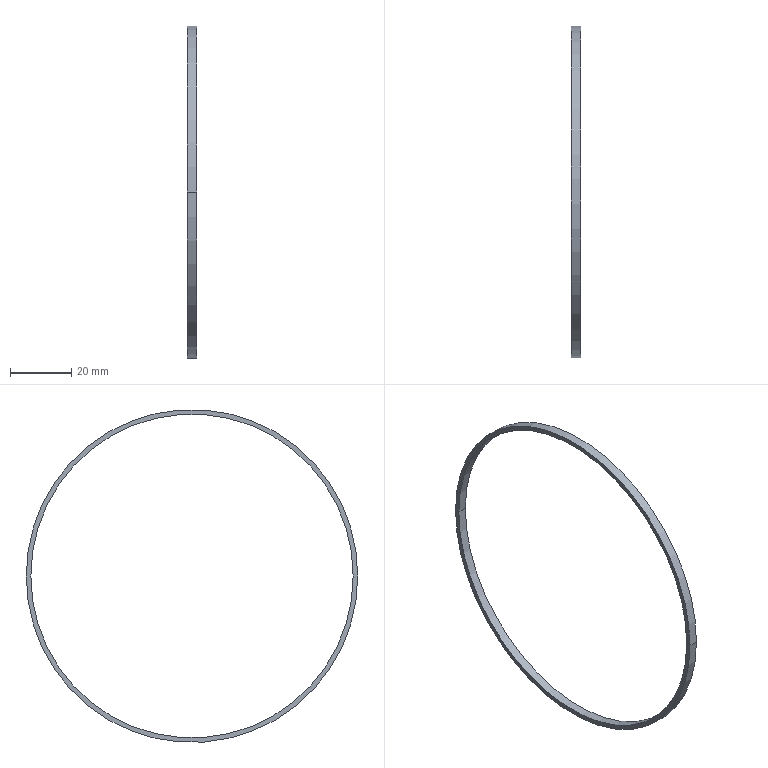Part | STEP file | 1-56.27 | 1 solid | 6 faces | box 3 x 108 x 108.5 mm | volume 1510 mm3 | cylinder 4 | plane 2 | commonest cylinder face diameters 105 x2 108 x2
STEP:
#1=CARTESIAN_POINT('',(0.,0.,0.));
#2=DIRECTION('',(0.,0.,1.));
#3=DIRECTION('',(1.,0.,0.));
#4=AXIS2_PLACEMENT_3D('',#1,#2,#3);
#5=CARTESIAN_POINT('',(0.,53.999,-0.25));
#6=VERTEX_POINT('',#5);
#7=CARTESIAN_POINT('',(0.,-53.999,-0.25));
#8=VERTEX_POINT('',#7);
#9=CARTESIAN_POINT('',(0.,0.,0.));
#10=DIRECTION('',(1.,0.,0.));
#11=DIRECTION('',(0.,1.,-0.00463));
#12=AXIS2_PLACEMENT_3D('',#9,#10,#11);
#13=CIRCLE('',#12,54.);
#14=CARTESIAN_POINT('',(0.,0.,-0.2494));
#15=DIRECTION('',(1.,0.,0.));
#16=DIRECTION('',(0.,1.,0.));
#17=AXIS2_PLACEMENT_3D('',#14,#15,#16);
#18=PLANE('',#17);
#19=CARTESIAN_POINT('',(0.,0.2494));
#20=DIRECTION('',(1.,-0.00463));
#21=AXIS2_PLACEMENT_2D('',#19,#20);
#22=CIRCLE('',#21,54.);
#23=(GEOMETRIC_REPRESENTATION_CONTEXT(2)PARAMETRIC_REPRESENTATION_CONTEXT()REPRESENTATION_CONTEXT('',''));
#24=DEFINITIONAL_REPRESENTATION('',(#22),#23);
#25=PCURVE('',#18,#24);
#26=CARTESIAN_POINT('',(0.,0.,0.));
#27=DIRECTION('',(1.,0.,0.));
#28=DIRECTION('',(0.,1.,-0.00463));
#29=AXIS2_PLACEMENT_3D('',#26,#27,#28);
#30=CYLINDRICAL_SURFACE('',#29,54.);
#31=CARTESIAN_POINT('',(0.,0.));
#32=DIRECTION('',(1.,0.));
#33=VECTOR('',#32,1.);
#34=LINE('',#31,#33);
#35=(GEOMETRIC_REPRESENTATION_CONTEXT(2)PARAMETRIC_REPRESENTATION_CONTEXT()REPRESENTATION_CONTEXT('',''));
#36=DEFINITIONAL_REPRESENTATION('',(#34),#35);
#37=PCURVE('',#30,#36);
#38=SURFACE_CURVE('',#13,(#25,#37),.PCURVE_S1.);
#39=EDGE_CURVE('',#6,#8,#38,.T.);
#40=ORIENTED_EDGE('',*,*,#39,.T.);
#41=CARTESIAN_POINT('',(0.,0.,-0.5));
#42=DIRECTION('',(1.,0.,0.));
#43=DIRECTION('',(0.,-1.,0.00463));
#44=AXIS2_PLACEMENT_3D('',#41,#42,#43);
#45=CIRCLE('',#44,54.);
#46=CARTESIAN_POINT('',(0.,-0.2506));
#47=DIRECTION('',(-1.,0.00463));
#48=AXIS2_PLACEMENT_2D('',#46,#47);
#49=CIRCLE('',#48,54.);
#50=(GEOMETRIC_REPRESENTATION_CONTEXT(2)PARAMETRIC_REPRESENTATION_CONTEXT()REPRESENTATION_CONTEXT('',''));
#51=DEFINITIONAL_REPRESENTATION('',(#49),#50);
#52=PCURVE('',#18,#51);
#53=CARTESIAN_POINT('',(0.,0.,-0.5));
#54=DIRECTION('',(1.,0.,0.));
#55=DIRECTION('',(0.,-1.,0.00463));
#56=AXIS2_PLACEMENT_3D('',#53,#54,#55);
#57=CYLINDRICAL_SURFACE('',#56,54.);
#58=CARTESIAN_POINT('',(0.,0.));
#59=DIRECTION('',(1.,0.));
#60=VECTOR('',#59,1.);
#61=LINE('',#58,#60);
#62=(GEOMETRIC_REPRESENTATION_CONTEXT(2)PARAMETRIC_REPRESENTATION_CONTEXT()REPRESENTATION_CONTEXT('',''));
#63=DEFINITIONAL_REPRESENTATION('',(#61),#62);
#64=PCURVE('',#57,#63);
#65=SURFACE_CURVE('',#45,(#52,#64),.PCURVE_S1.);
#66=EDGE_CURVE('',#8,#6,#65,.T.);
#67=ORIENTED_EDGE('',*,*,#66,.T.);
#68=EDGE_LOOP('',(#40,#67));
#69=FACE_BOUND('',#68,.F.);
#70=CARTESIAN_POINT('',(0.,52.499,-0.25));
#71=VERTEX_POINT('',#70);
#72=CARTESIAN_POINT('',(0.,-52.499,-0.25));
#73=VERTEX_POINT('',#72);
#74=CARTESIAN_POINT('',(0.,0.,-0.5));
#75=DIRECTION('',(-1.,0.,0.));
#76=DIRECTION('',(0.,1.,0.004762));
#77=AXIS2_PLACEMENT_3D('',#74,#75,#76);
#78=CIRCLE('',#77,52.5);
#79=CARTESIAN_POINT('',(52.499,-0.0005814));
#80=CARTESIAN_POINT('',(52.932,-90.932));
#81=CARTESIAN_POINT('',(-26.033,-45.841));
#82=CARTESIAN_POINT('',(-104.999,-0.7506));
#83=CARTESIAN_POINT('',(-26.466,45.09));
#84=CARTESIAN_POINT('',(52.066,90.931));
#85=CARTESIAN_POINT('',(52.499,-0.0005814));
#86=(BOUNDED_CURVE()B_SPLINE_CURVE(2,(#79,#80,#81,#82,#83,#84,#85),.UNSPECIFIED.,.T.,.F.)B_SPLINE_CURVE_WITH_KNOTS((1,2,2,2,2,1),(-2.094,0.,2.094,4.189,6.283,8.378),.UNSPECIFIED.)CURVE()GEOMETRIC_REPRESENTATION_ITEM()RATIONAL_B_SPLINE_CURVE((1.,0.5,1.,0.5,1.,0.5,1.))REPRESENTATION_ITEM(''));
#87=(GEOMETRIC_REPRESENTATION_CONTEXT(2)PARAMETRIC_REPRESENTATION_CONTEXT()REPRESENTATION_CONTEXT('',''));
#88=DEFINITIONAL_REPRESENTATION('',(#86),#87);
#89=PCURVE('',#18,#88);
#90=CARTESIAN_POINT('',(0.,0.,-0.5));
#91=DIRECTION('',(1.,0.,0.));
#92=DIRECTION('',(0.,1.,0.004762));
#93=AXIS2_PLACEMENT_3D('',#90,#91,#92);
#94=CYLINDRICAL_SURFACE('',#93,52.5);
#95=CARTESIAN_POINT('',(6.283,0.));
#96=DIRECTION('',(-1.,0.));
#97=VECTOR('',#96,1.);
#98=LINE('',#95,#97);
#99=(GEOMETRIC_REPRESENTATION_CONTEXT(2)PARAMETRIC_REPRESENTATION_CONTEXT()REPRESENTATION_CONTEXT('',''));
#100=DEFINITIONAL_REPRESENTATION('',(#98),#99);
#101=PCURVE('',#94,#100);
#102=SURFACE_CURVE('',#78,(#89,#101),.PCURVE_S1.);
#103=EDGE_CURVE('',#71,#73,#102,.T.);
#104=ORIENTED_EDGE('',*,*,#103,.T.);
#105=CARTESIAN_POINT('',(0.,0.,0.));
#106=DIRECTION('',(-1.,0.,0.));
#107=DIRECTION('',(0.,-1.,-0.004762));
#108=AXIS2_PLACEMENT_3D('',#105,#106,#107);
#109=CIRCLE('',#108,52.5);
#110=CARTESIAN_POINT('',(-52.499,-0.0005814));
#111=CARTESIAN_POINT('',(-52.932,90.931));
#112=CARTESIAN_POINT('',(26.033,45.84));
#113=CARTESIAN_POINT('',(104.999,0.7494));
#114=CARTESIAN_POINT('',(26.466,-45.091));
#115=CARTESIAN_POINT('',(-52.066,-90.932));
#116=CARTESIAN_POINT('',(-52.499,-0.0005814));
#117=(BOUNDED_CURVE()B_SPLINE_CURVE(2,(#110,#111,#112,#113,#114,#115,#116),.UNSPECIFIED.,.T.,.F.)B_SPLINE_CURVE_WITH_KNOTS((1,2,2,2,2,1),(-2.094,0.,2.094,4.189,6.283,8.378),.UNSPECIFIED.)CURVE()GEOMETRIC_REPRESENTATION_ITEM()RATIONAL_B_SPLINE_CURVE((1.,0.5,1.,0.5,1.,0.5,1.))REPRESENTATION_ITEM(''));
#118=(GEOMETRIC_REPRESENTATION_CONTEXT(2)PARAMETRIC_REPRESENTATION_CONTEXT()REPRESENTATION_CONTEXT('',''));
#119=DEFINITIONAL_REPRESENTATION('',(#117),#118);
#120=PCURVE('',#18,#119);
#121=CARTESIAN_POINT('',(0.,0.,0.));
#122=DIRECTION('',(1.,0.,0.));
#123=DIRECTION('',(0.,-1.,-0.004762));
#124=AXIS2_PLACEMENT_3D('',#121,#122,#123);
#125=CYLINDRICAL_SURFACE('',#124,52.5);
#126=CARTESIAN_POINT('',(6.283,0.));
#127=DIRECTION('',(-1.,0.));
#128=VECTOR('',#127,1.);
#129=LINE('',#126,#128);
#130=(GEOMETRIC_REPRESENTATION_CONTEXT(2)PARAMETRIC_REPRESENTATION_CONTEXT()REPRESENTATION_CONTEXT('',''));
#131=DEFINITIONAL_REPRESENTATION('',(#129),#130);
#132=PCURVE('',#125,#131);
#133=SURFACE_CURVE('',#109,(#120,#132),.PCURVE_S1.);
#134=EDGE_CURVE('',#73,#71,#133,.T.);
#135=ORIENTED_EDGE('',*,*,#134,.T.);
#136=EDGE_LOOP('',(#104,#135));
#137=FACE_BOUND('',#136,.F.);
#138=ADVANCED_FACE('',(#69,#137),#18,.F.);
#139=CARTESIAN_POINT('',(3.,53.999,-0.25));
#140=VERTEX_POINT('',#139);
#141=CARTESIAN_POINT('',(3.,-53.999,-0.25));
#142=VERTEX_POINT('',#141);
#143=CARTESIAN_POINT('',(3.,0.,0.));
#144=DIRECTION('',(1.,0.,0.));
#145=DIRECTION('',(0.,1.,-0.00463));
#146=AXIS2_PLACEMENT_3D('',#143,#144,#145);
#147=CIRCLE('',#146,54.);
#148=CARTESIAN_POINT('',(3.,0.,-0.2494));
#149=DIRECTION('',(1.,0.,0.));
#150=DIRECTION('',(0.,1.,0.));
#151=AXIS2_PLACEMENT_3D('',#148,#149,#150);
#152=PLANE('',#151);
#153=CARTESIAN_POINT('',(0.,0.2494));
#154=DIRECTION('',(1.,-0.00463));
#155=AXIS2_PLACEMENT_2D('',#153,#154);
#156=CIRCLE('',#155,54.);
#157=(GEOMETRIC_REPRESENTATION_CONTEXT(2)PARAMETRIC_REPRESENTATION_CONTEXT()REPRESENTATION_CONTEXT('',''));
#158=DEFINITIONAL_REPRESENTATION('',(#156),#157);
#159=PCURVE('',#152,#158);
#160=CARTESIAN_POINT('',(0.,3.));
#161=DIRECTION('',(1.,0.));
#162=VECTOR('',#161,1.);
#163=LINE('',#160,#162);
#164=(GEOMETRIC_REPRESENTATION_CONTEXT(2)PARAMETRIC_REPRESENTATION_CONTEXT()REPRESENTATION_CONTEXT('',''));
#165=DEFINITIONAL_REPRESENTATION('',(#163),#164);
#166=PCURVE('',#30,#165);
#167=SURFACE_CURVE('',#147,(#159,#166),.PCURVE_S1.);
#168=EDGE_CURVE('',#140,#142,#167,.T.);
#169=ORIENTED_EDGE('',*,*,#168,.T.);
#170=CARTESIAN_POINT('',(3.,0.,-0.5));
#171=DIRECTION('',(1.,0.,0.));
#172=DIRECTION('',(0.,-1.,0.00463));
#173=AXIS2_PLACEMENT_3D('',#170,#171,#172);
#174=CIRCLE('',#173,54.);
#175=CARTESIAN_POINT('',(0.,-0.2506));
#176=DIRECTION('',(-1.,0.00463));
#177=AXIS2_PLACEMENT_2D('',#175,#176);
#178=CIRCLE('',#177,54.);
#179=(GEOMETRIC_REPRESENTATION_CONTEXT(2)PARAMETRIC_REPRESENTATION_CONTEXT()REPRESENTATION_CONTEXT('',''));
#180=DEFINITIONAL_REPRESENTATION('',(#178),#179);
#181=PCURVE('',#152,#180);
#182=CARTESIAN_POINT('',(0.,3.));
#183=DIRECTION('',(1.,0.));
#184=VECTOR('',#183,1.);
#185=LINE('',#182,#184);
#186=(GEOMETRIC_REPRESENTATION_CONTEXT(2)PARAMETRIC_REPRESENTATION_CONTEXT()REPRESENTATION_CONTEXT('',''));
#187=DEFINITIONAL_REPRESENTATION('',(#185),#186);
#188=PCURVE('',#57,#187);
#189=SURFACE_CURVE('',#174,(#181,#188),.PCURVE_S1.);
#190=EDGE_CURVE('',#142,#140,#189,.T.);
#191=ORIENTED_EDGE('',*,*,#190,.T.);
#192=EDGE_LOOP('',(#169,#191));
#193=FACE_BOUND('',#192,.T.);
#194=CARTESIAN_POINT('',(3.,52.499,-0.25));
#195=VERTEX_POINT('',#194);
#196=CARTESIAN_POINT('',(3.,-52.499,-0.25));
#197=VERTEX_POINT('',#196);
#198=CARTESIAN_POINT('',(3.,0.,-0.5));
#199=DIRECTION('',(-1.,0.,0.));
#200=DIRECTION('',(0.,1.,0.004762));
#201=AXIS2_PLACEMENT_3D('',#198,#199,#200);
#202=CIRCLE('',#201,52.5);
#203=CARTESIAN_POINT('',(52.499,-0.0005814));
#204=CARTESIAN_POINT('',(52.932,-90.932));
#205=CARTESIAN_POINT('',(-26.033,-45.841));
#206=CARTESIAN_POINT('',(-104.999,-0.7506));
#207=CARTESIAN_POINT('',(-26.466,45.09));
#208=CARTESIAN_POINT('',(52.066,90.931));
#209=CARTESIAN_POINT('',(52.499,-0.0005814));
#210=(BOUNDED_CURVE()B_SPLINE_CURVE(2,(#203,#204,#205,#206,#207,#208,#209),.UNSPECIFIED.,.T.,.F.)B_SPLINE_CURVE_WITH_KNOTS((1,2,2,2,2,1),(-2.094,0.,2.094,4.189,6.283,8.378),.UNSPECIFIED.)CURVE()GEOMETRIC_REPRESENTATION_ITEM()RATIONAL_B_SPLINE_CURVE((1.,0.5,1.,0.5,1.,0.5,1.))REPRESENTATION_ITEM(''));
#211=(GEOMETRIC_REPRESENTATION_CONTEXT(2)PARAMETRIC_REPRESENTATION_CONTEXT()REPRESENTATION_CONTEXT('',''));
#212=DEFINITIONAL_REPRESENTATION('',(#210),#211);
#213=PCURVE('',#152,#212);
#214=CARTESIAN_POINT('',(6.283,3.));
#215=DIRECTION('',(-1.,0.));
#216=VECTOR('',#215,1.);
#217=LINE('',#214,#216);
#218=(GEOMETRIC_REPRESENTATION_CONTEXT(2)PARAMETRIC_REPRESENTATION_CONTEXT()REPRESENTATION_CONTEXT('',''));
#219=DEFINITIONAL_REPRESENTATION('',(#217),#218);
#220=PCURVE('',#94,#219);
#221=SURFACE_CURVE('',#202,(#213,#220),.PCURVE_S1.);
#222=EDGE_CURVE('',#195,#197,#221,.T.);
#223=ORIENTED_EDGE('',*,*,#222,.T.);
#224=CARTESIAN_POINT('',(3.,0.,0.));
#225=DIRECTION('',(-1.,0.,0.));
#226=DIRECTION('',(0.,-1.,-0.004762));
#227=AXIS2_PLACEMENT_3D('',#224,#225,#226);
#228=CIRCLE('',#227,52.5);
#229=CARTESIAN_POINT('',(-52.499,-0.0005814));
#230=CARTESIAN_POINT('',(-52.932,90.931));
#231=CARTESIAN_POINT('',(26.033,45.84));
#232=CARTESIAN_POINT('',(104.999,0.7494));
#233=CARTESIAN_POINT('',(26.466,-45.091));
#234=CARTESIAN_POINT('',(-52.066,-90.932));
#235=CARTESIAN_POINT('',(-52.499,-0.0005814));
#236=(BOUNDED_CURVE()B_SPLINE_CURVE(2,(#229,#230,#231,#232,#233,#234,#235),.UNSPECIFIED.,.T.,.F.)B_SPLINE_CURVE_WITH_KNOTS((1,2,2,2,2,1),(-2.094,0.,2.094,4.189,6.283,8.378),.UNSPECIFIED.)CURVE()GEOMETRIC_REPRESENTATION_ITEM()RATIONAL_B_SPLINE_CURVE((1.,0.5,1.,0.5,1.,0.5,1.))REPRESENTATION_ITEM(''));
#237=(GEOMETRIC_REPRESENTATION_CONTEXT(2)PARAMETRIC_REPRESENTATION_CONTEXT()REPRESENTATION_CONTEXT('',''));
#238=DEFINITIONAL_REPRESENTATION('',(#236),#237);
#239=PCURVE('',#152,#238);
#240=CARTESIAN_POINT('',(6.283,3.));
#241=DIRECTION('',(-1.,0.));
#242=VECTOR('',#241,1.);
#243=LINE('',#240,#242);
#244=(GEOMETRIC_REPRESENTATION_CONTEXT(2)PARAMETRIC_REPRESENTATION_CONTEXT()REPRESENTATION_CONTEXT('',''));
#245=DEFINITIONAL_REPRESENTATION('',(#243),#244);
#246=PCURVE('',#125,#245);
#247=SURFACE_CURVE('',#228,(#239,#246),.PCURVE_S1.);
#248=EDGE_CURVE('',#197,#195,#247,.T.);
#249=ORIENTED_EDGE('',*,*,#248,.T.);
#250=EDGE_LOOP('',(#223,#249));
#251=FACE_BOUND('',#250,.T.);
#252=ADVANCED_FACE('',(#193,#251),#152,.T.);
#253=ORIENTED_EDGE('',*,*,#39,.T.);
#254=CARTESIAN_POINT('',(0.,-53.999,-0.25));
#255=DIRECTION('',(1.,0.,0.));
#256=VECTOR('',#255,1.);
#257=LINE('',#254,#256);
#258=CARTESIAN_POINT('',(3.151,0.));
#259=DIRECTION('',(0.,1.));
#260=VECTOR('',#259,1.);
#261=LINE('',#258,#260);
#262=(GEOMETRIC_REPRESENTATION_CONTEXT(2)PARAMETRIC_REPRESENTATION_CONTEXT()REPRESENTATION_CONTEXT('',''));
#263=DEFINITIONAL_REPRESENTATION('',(#261),#262);
#264=PCURVE('',#30,#263);
#265=CARTESIAN_POINT('',(0.,0.));
#266=DIRECTION('',(0.,1.));
#267=VECTOR('',#266,1.);
#268=LINE('',#265,#267);
#269=(GEOMETRIC_REPRESENTATION_CONTEXT(2)PARAMETRIC_REPRESENTATION_CONTEXT()REPRESENTATION_CONTEXT('',''));
#270=DEFINITIONAL_REPRESENTATION('',(#268),#269);
#271=PCURVE('',#57,#270);
#272=SURFACE_CURVE('',#257,(#264,#271),.PCURVE_S1.);
#273=EDGE_CURVE('',#8,#142,#272,.T.);
#274=ORIENTED_EDGE('',*,*,#273,.T.);
#275=ORIENTED_EDGE('',*,*,#168,.F.);
#276=CARTESIAN_POINT('',(0.,53.999,-0.25));
#277=DIRECTION('',(1.,0.,0.));
#278=VECTOR('',#277,1.);
#279=LINE('',#276,#278);
#280=CARTESIAN_POINT('',(0.,0.));
#281=DIRECTION('',(0.,1.));
#282=VECTOR('',#281,1.);
#283=LINE('',#280,#282);
#284=(GEOMETRIC_REPRESENTATION_CONTEXT(2)PARAMETRIC_REPRESENTATION_CONTEXT()REPRESENTATION_CONTEXT('',''));
#285=DEFINITIONAL_REPRESENTATION('',(#283),#284);
#286=PCURVE('',#30,#285);
#287=CARTESIAN_POINT('',(3.151,0.));
#288=DIRECTION('',(0.,1.));
#289=VECTOR('',#288,1.);
#290=LINE('',#287,#289);
#291=(GEOMETRIC_REPRESENTATION_CONTEXT(2)PARAMETRIC_REPRESENTATION_CONTEXT()REPRESENTATION_CONTEXT('',''));
#292=DEFINITIONAL_REPRESENTATION('',(#290),#291);
#293=PCURVE('',#57,#292);
#294=SURFACE_CURVE('',#279,(#286,#293),.PCURVE_S1.);
#295=EDGE_CURVE('',#6,#140,#294,.T.);
#296=ORIENTED_EDGE('',*,*,#295,.F.);
#297=EDGE_LOOP('',(#253,#274,#275,#296));
#298=FACE_BOUND('',#297,.T.);
#299=ADVANCED_FACE('',(#298),#30,.T.);
#300=ORIENTED_EDGE('',*,*,#66,.T.);
#301=ORIENTED_EDGE('',*,*,#295,.T.);
#302=ORIENTED_EDGE('',*,*,#190,.F.);
#303=ORIENTED_EDGE('',*,*,#273,.F.);
#304=EDGE_LOOP('',(#300,#301,#302,#303));
#305=FACE_BOUND('',#304,.T.);
#306=ADVANCED_FACE('',(#305),#57,.T.);
#307=CARTESIAN_POINT('',(0.,52.499,-0.25));
#308=DIRECTION('',(1.,0.,0.));
#309=VECTOR('',#308,1.);
#310=LINE('',#307,#309);
#311=CARTESIAN_POINT('',(6.283,0.));
#312=DIRECTION('',(0.,1.));
#313=VECTOR('',#312,1.);
#314=LINE('',#311,#313);
#315=(GEOMETRIC_REPRESENTATION_CONTEXT(2)PARAMETRIC_REPRESENTATION_CONTEXT()REPRESENTATION_CONTEXT('',''));
#316=DEFINITIONAL_REPRESENTATION('',(#314),#315);
#317=PCURVE('',#94,#316);
#318=CARTESIAN_POINT('',(3.132,0.));
#319=DIRECTION('',(0.,1.));
#320=VECTOR('',#319,1.);
#321=LINE('',#318,#320);
#322=(GEOMETRIC_REPRESENTATION_CONTEXT(2)PARAMETRIC_REPRESENTATION_CONTEXT()REPRESENTATION_CONTEXT('',''));
#323=DEFINITIONAL_REPRESENTATION('',(#321),#322);
#324=PCURVE('',#125,#323);
#325=SURFACE_CURVE('',#310,(#317,#324),.PCURVE_S1.);
#326=EDGE_CURVE('',#71,#195,#325,.T.);
#327=ORIENTED_EDGE('',*,*,#326,.T.);
#328=ORIENTED_EDGE('',*,*,#222,.T.);
#329=CARTESIAN_POINT('',(0.,-52.499,-0.25));
#330=DIRECTION('',(1.,0.,0.));
#331=VECTOR('',#330,1.);
#332=LINE('',#329,#331);
#333=CARTESIAN_POINT('',(3.132,0.));
#334=DIRECTION('',(0.,1.));
#335=VECTOR('',#334,1.);
#336=LINE('',#333,#335);
#337=(GEOMETRIC_REPRESENTATION_CONTEXT(2)PARAMETRIC_REPRESENTATION_CONTEXT()REPRESENTATION_CONTEXT('',''));
#338=DEFINITIONAL_REPRESENTATION('',(#336),#337);
#339=PCURVE('',#94,#338);
#340=CARTESIAN_POINT('',(6.283,0.));
#341=DIRECTION('',(0.,1.));
#342=VECTOR('',#341,1.);
#343=LINE('',#340,#342);
#344=(GEOMETRIC_REPRESENTATION_CONTEXT(2)PARAMETRIC_REPRESENTATION_CONTEXT()REPRESENTATION_CONTEXT('',''));
#345=DEFINITIONAL_REPRESENTATION('',(#343),#344);
#346=PCURVE('',#125,#345);
#347=SURFACE_CURVE('',#332,(#339,#346),.PCURVE_S1.);
#348=EDGE_CURVE('',#73,#197,#347,.T.);
#349=ORIENTED_EDGE('',*,*,#348,.F.);
#350=ORIENTED_EDGE('',*,*,#103,.F.);
#351=EDGE_LOOP('',(#327,#328,#349,#350));
#352=FACE_BOUND('',#351,.F.);
#353=ADVANCED_FACE('',(#352),#94,.F.);
#354=ORIENTED_EDGE('',*,*,#348,.T.);
#355=ORIENTED_EDGE('',*,*,#248,.T.);
#356=ORIENTED_EDGE('',*,*,#326,.F.);
#357=ORIENTED_EDGE('',*,*,#134,.F.);
#358=EDGE_LOOP('',(#354,#355,#356,#357));
#359=FACE_BOUND('',#358,.F.);
#360=ADVANCED_FACE('',(#359),#125,.F.);
#361=CLOSED_SHELL('',(#138,#252,#299,#306,#353,#360));
#362=MANIFOLD_SOLID_BREP('',#361);
#363=(LENGTH_UNIT()NAMED_UNIT(*)SI_UNIT(.MILLI.,.METRE.));
#364=UNCERTAINTY_MEASURE_WITH_UNIT(LENGTH_MEASURE(0.0000001),#363,'','');
#365=(NAMED_UNIT(*)PLANE_ANGLE_UNIT()SI_UNIT($,.RADIAN.));
#366=(NAMED_UNIT(*)SI_UNIT($,.STERADIAN.)SOLID_ANGLE_UNIT());
#367=(GEOMETRIC_REPRESENTATION_CONTEXT(3)GLOBAL_UNCERTAINTY_ASSIGNED_CONTEXT((#364))GLOBAL_UNIT_ASSIGNED_CONTEXT((#363,#365,#366))REPRESENTATION_CONTEXT('',''));
#368=ADVANCED_BREP_SHAPE_REPRESENTATION('',(#4,#362),#367);